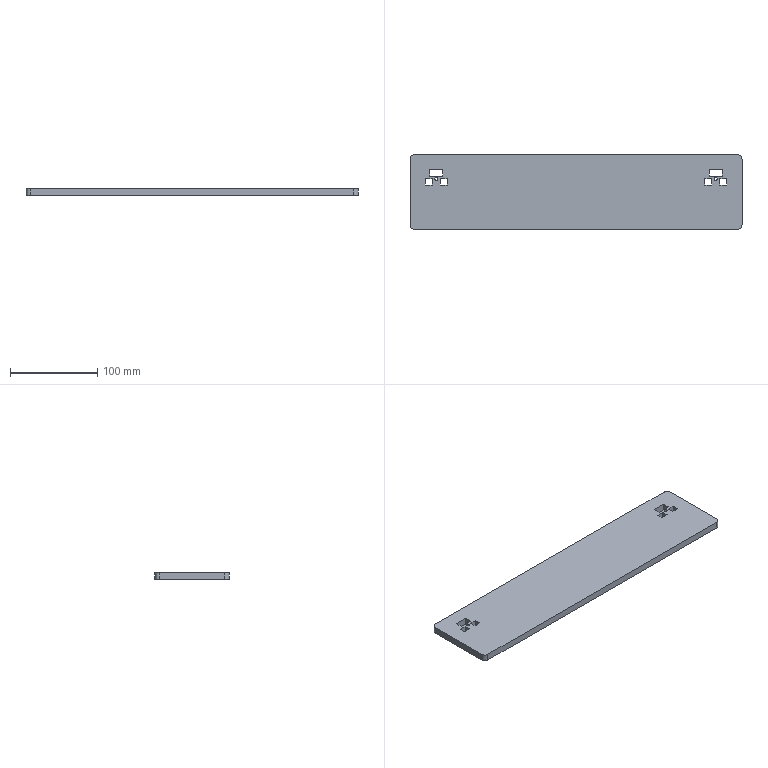Part | SolidWorks | features Fillet 1, FlatPattern 1, SMBaseFlange 1, SheetMetal 1 | 1 solid | 38 faces | box 380 x 85 x 8 mm | volume 254362 mm3 | plane 30 | cylinder 8 | commonest cylinder face diameters 3.5 x4 10 x4
STEP:
#1=CARTESIAN_POINT('',(322.8,26.043,8.));
#2=VERTEX_POINT('',#1);
#3=CARTESIAN_POINT('',(326.3,26.043,8.));
#4=VERTEX_POINT('',#3);
#5=CARTESIAN_POINT('',(324.55,26.043,8.));
#6=DIRECTION('',(0.,0.,1.));
#7=DIRECTION('',(1.,0.,0.));
#8=AXIS2_PLACEMENT_3D('',#5,#6,#7);
#9=CIRCLE('',#8,1.75);
#10=EDGE_CURVE('',#2,#4,#9,.T.);
#11=ORIENTED_EDGE('',*,*,#10,.T.);
#12=CARTESIAN_POINT('',(326.3,26.043,0.));
#13=VERTEX_POINT('',#12);
#14=CARTESIAN_POINT('',(326.3,26.043,8.));
#15=DIRECTION('',(0.,0.,-1.));
#16=VECTOR('',#15,1000.);
#17=LINE('',#14,#16);
#18=EDGE_CURVE('',#4,#13,#17,.T.);
#19=ORIENTED_EDGE('',*,*,#18,.T.);
#20=CARTESIAN_POINT('',(322.8,26.043,0.));
#21=VERTEX_POINT('',#20);
#22=CARTESIAN_POINT('',(324.55,26.043,0.));
#23=DIRECTION('',(0.,0.,1.));
#24=DIRECTION('',(1.,0.,0.));
#25=AXIS2_PLACEMENT_3D('',#22,#23,#24);
#26=CIRCLE('',#25,1.75);
#27=EDGE_CURVE('',#21,#13,#26,.T.);
#28=ORIENTED_EDGE('',*,*,#27,.F.);
#29=CARTESIAN_POINT('',(322.8,26.043,8.));
#30=DIRECTION('',(0.,0.,-1.));
#31=VECTOR('',#30,1000.);
#32=LINE('',#29,#31);
#33=EDGE_CURVE('',#2,#21,#32,.T.);
#34=ORIENTED_EDGE('',*,*,#33,.F.);
#35=EDGE_LOOP('',(#11,#19,#28,#34));
#36=FACE_OUTER_BOUND('',#35,.T.);
#37=CARTESIAN_POINT('',(324.55,26.043,8.));
#38=DIRECTION('',(0.,0.,-1.));
#39=DIRECTION('',(-1.,0.,0.));
#40=AXIS2_PLACEMENT_3D('',#37,#38,#39);
#41=CYLINDRICAL_SURFACE('',#40,1.75);
#42=ADVANCED_FACE('',(#36),#41,.F.);
#43=CARTESIAN_POINT('',(2.8,26.043,8.));
#44=VERTEX_POINT('',#43);
#45=CARTESIAN_POINT('',(6.3,26.043,8.));
#46=VERTEX_POINT('',#45);
#47=CARTESIAN_POINT('',(4.55,26.043,8.));
#48=DIRECTION('',(0.,0.,1.));
#49=DIRECTION('',(1.,0.,0.));
#50=AXIS2_PLACEMENT_3D('',#47,#48,#49);
#51=CIRCLE('',#50,1.75);
#52=EDGE_CURVE('',#44,#46,#51,.T.);
#53=ORIENTED_EDGE('',*,*,#52,.T.);
#54=CARTESIAN_POINT('',(6.3,26.043,0.));
#55=VERTEX_POINT('',#54);
#56=CARTESIAN_POINT('',(6.3,26.043,8.));
#57=DIRECTION('',(0.,0.,-1.));
#58=VECTOR('',#57,1000.);
#59=LINE('',#56,#58);
#60=EDGE_CURVE('',#46,#55,#59,.T.);
#61=ORIENTED_EDGE('',*,*,#60,.T.);
#62=CARTESIAN_POINT('',(2.8,26.043,0.));
#63=VERTEX_POINT('',#62);
#64=CARTESIAN_POINT('',(4.55,26.043,0.));
#65=DIRECTION('',(0.,0.,1.));
#66=DIRECTION('',(1.,0.,0.));
#67=AXIS2_PLACEMENT_3D('',#64,#65,#66);
#68=CIRCLE('',#67,1.75);
#69=EDGE_CURVE('',#63,#55,#68,.T.);
#70=ORIENTED_EDGE('',*,*,#69,.F.);
#71=CARTESIAN_POINT('',(2.8,26.043,8.));
#72=DIRECTION('',(0.,0.,-1.));
#73=VECTOR('',#72,1000.);
#74=LINE('',#71,#73);
#75=EDGE_CURVE('',#44,#63,#74,.T.);
#76=ORIENTED_EDGE('',*,*,#75,.F.);
#77=EDGE_LOOP('',(#53,#61,#70,#76));
#78=FACE_OUTER_BOUND('',#77,.T.);
#79=CARTESIAN_POINT('',(4.55,26.043,8.));
#80=DIRECTION('',(0.,0.,-1.));
#81=DIRECTION('',(-1.,0.,0.));
#82=AXIS2_PLACEMENT_3D('',#79,#80,#81);
#83=CYLINDRICAL_SURFACE('',#82,1.75);
#84=ADVANCED_FACE('',(#78),#83,.F.);
#85=CARTESIAN_POINT('',(320.,19.043,8.));
#86=VERTEX_POINT('',#85);
#87=CARTESIAN_POINT('',(320.,26.043,8.));
#88=VERTEX_POINT('',#87);
#89=CARTESIAN_POINT('',(320.,26.043,8.));
#90=DIRECTION('',(0.,1.,0.));
#91=VECTOR('',#90,1000.);
#92=LINE('',#89,#91);
#93=EDGE_CURVE('',#86,#88,#92,.T.);
#94=ORIENTED_EDGE('',*,*,#93,.F.);
#95=CARTESIAN_POINT('',(312.,19.043,8.));
#96=VERTEX_POINT('',#95);
#97=CARTESIAN_POINT('',(320.,19.043,8.));
#98=DIRECTION('',(1.,0.,0.));
#99=VECTOR('',#98,1000.);
#100=LINE('',#97,#99);
#101=EDGE_CURVE('',#96,#86,#100,.T.);
#102=ORIENTED_EDGE('',*,*,#101,.F.);
#103=CARTESIAN_POINT('',(312.,26.043,8.));
#104=VERTEX_POINT('',#103);
#105=CARTESIAN_POINT('',(312.,26.043,8.));
#106=DIRECTION('',(0.,-1.,0.));
#107=VECTOR('',#106,1000.);
#108=LINE('',#105,#107);
#109=EDGE_CURVE('',#104,#96,#108,.T.);
#110=ORIENTED_EDGE('',*,*,#109,.F.);
#111=CARTESIAN_POINT('',(320.,26.043,8.));
#112=DIRECTION('',(-1.,0.,0.));
#113=VECTOR('',#112,1000.);
#114=LINE('',#111,#113);
#115=EDGE_CURVE('',#88,#104,#114,.T.);
#116=ORIENTED_EDGE('',*,*,#115,.F.);
#117=EDGE_LOOP('',(#94,#102,#110,#116));
#118=FACE_BOUND('',#117,.T.);
#119=CARTESIAN_POINT('',(-8.,26.043,8.));
#120=VERTEX_POINT('',#119);
#121=CARTESIAN_POINT('',(-8.,19.043,8.));
#122=VERTEX_POINT('',#121);
#123=CARTESIAN_POINT('',(-8.,19.043,8.));
#124=DIRECTION('',(0.,-1.,0.));
#125=VECTOR('',#124,1000.);
#126=LINE('',#123,#125);
#127=EDGE_CURVE('',#120,#122,#126,.T.);
#128=ORIENTED_EDGE('',*,*,#127,.F.);
#129=CARTESIAN_POINT('',(0.,26.043,8.));
#130=VERTEX_POINT('',#129);
#131=CARTESIAN_POINT('',(-8.,26.043,8.));
#132=DIRECTION('',(-1.,0.,0.));
#133=VECTOR('',#132,1000.);
#134=LINE('',#131,#133);
#135=EDGE_CURVE('',#130,#120,#134,.T.);
#136=ORIENTED_EDGE('',*,*,#135,.F.);
#137=CARTESIAN_POINT('',(0.,19.043,8.));
#138=VERTEX_POINT('',#137);
#139=CARTESIAN_POINT('',(0.,19.043,8.));
#140=DIRECTION('',(0.,1.,0.));
#141=VECTOR('',#140,1000.);
#142=LINE('',#139,#141);
#143=EDGE_CURVE('',#138,#130,#142,.T.);
#144=ORIENTED_EDGE('',*,*,#143,.F.);
#145=CARTESIAN_POINT('',(-8.,19.043,8.));
#146=DIRECTION('',(1.,0.,0.));
#147=VECTOR('',#146,1000.);
#148=LINE('',#145,#147);
#149=EDGE_CURVE('',#122,#138,#148,.T.);
#150=ORIENTED_EDGE('',*,*,#149,.F.);
#151=EDGE_LOOP('',(#128,#136,#144,#150));
#152=FACE_BOUND('',#151,.T.);
#153=CARTESIAN_POINT('',(-2.95,37.043,8.));
#154=VERTEX_POINT('',#153);
#155=CARTESIAN_POINT('',(-2.95,29.043,8.));
#156=VERTEX_POINT('',#155);
#157=CARTESIAN_POINT('',(-2.95,29.043,8.));
#158=DIRECTION('',(0.,-1.,0.));
#159=VECTOR('',#158,1000.);
#160=LINE('',#157,#159);
#161=EDGE_CURVE('',#154,#156,#160,.T.);
#162=ORIENTED_EDGE('',*,*,#161,.F.);
#163=CARTESIAN_POINT('',(12.05,37.043,8.));
#164=VERTEX_POINT('',#163);
#165=CARTESIAN_POINT('',(-2.95,37.043,8.));
#166=DIRECTION('',(-1.,0.,0.));
#167=VECTOR('',#166,1000.);
#168=LINE('',#165,#167);
#169=EDGE_CURVE('',#164,#154,#168,.T.);
#170=ORIENTED_EDGE('',*,*,#169,.F.);
#171=CARTESIAN_POINT('',(12.05,29.043,8.));
#172=VERTEX_POINT('',#171);
#173=CARTESIAN_POINT('',(12.05,29.043,8.));
#174=DIRECTION('',(0.,1.,0.));
#175=VECTOR('',#174,1000.);
#176=LINE('',#173,#175);
#177=EDGE_CURVE('',#172,#164,#176,.T.);
#178=ORIENTED_EDGE('',*,*,#177,.F.);
#179=CARTESIAN_POINT('',(-2.95,29.043,8.));
#180=DIRECTION('',(1.,0.,0.));
#181=VECTOR('',#180,1000.);
#182=LINE('',#179,#181);
#183=EDGE_CURVE('',#156,#172,#182,.T.);
#184=ORIENTED_EDGE('',*,*,#183,.F.);
#185=EDGE_LOOP('',(#162,#170,#178,#184));
#186=FACE_BOUND('',#185,.T.);
#187=CARTESIAN_POINT('',(354.55,-26.457,8.));
#188=VERTEX_POINT('',#187);
#189=CARTESIAN_POINT('',(354.55,48.543,8.));
#190=VERTEX_POINT('',#189);
#191=CARTESIAN_POINT('',(354.55,-31.457,8.));
#192=DIRECTION('',(0.,1.,0.));
#193=VECTOR('',#192,1000.);
#194=LINE('',#191,#193);
#195=EDGE_CURVE('',#188,#190,#194,.T.);
#196=ORIENTED_EDGE('',*,*,#195,.T.);
#197=CARTESIAN_POINT('',(349.55,53.543,8.));
#198=VERTEX_POINT('',#197);
#199=CARTESIAN_POINT('',(349.55,48.543,8.));
#200=DIRECTION('',(0.,0.,1.));
#201=DIRECTION('',(-1.,0.,0.));
#202=AXIS2_PLACEMENT_3D('',#199,#200,#201);
#203=CIRCLE('',#202,5.);
#204=EDGE_CURVE('',#190,#198,#203,.T.);
#205=ORIENTED_EDGE('',*,*,#204,.T.);
#206=CARTESIAN_POINT('',(-20.45,53.543,8.));
#207=VERTEX_POINT('',#206);
#208=CARTESIAN_POINT('',(-25.45,53.543,8.));
#209=DIRECTION('',(-1.,0.,0.));
#210=VECTOR('',#209,1000.);
#211=LINE('',#208,#210);
#212=EDGE_CURVE('',#198,#207,#211,.T.);
#213=ORIENTED_EDGE('',*,*,#212,.T.);
#214=CARTESIAN_POINT('',(-25.45,48.543,8.));
#215=VERTEX_POINT('',#214);
#216=CARTESIAN_POINT('',(-20.45,48.543,8.));
#217=DIRECTION('',(0.,0.,1.));
#218=DIRECTION('',(-1.,0.,0.));
#219=AXIS2_PLACEMENT_3D('',#216,#217,#218);
#220=CIRCLE('',#219,5.);
#221=EDGE_CURVE('',#207,#215,#220,.T.);
#222=ORIENTED_EDGE('',*,*,#221,.T.);
#223=CARTESIAN_POINT('',(-25.45,-26.457,8.));
#224=VERTEX_POINT('',#223);
#225=CARTESIAN_POINT('',(-25.45,-31.457,8.));
#226=DIRECTION('',(0.,-1.,0.));
#227=VECTOR('',#226,1000.);
#228=LINE('',#225,#227);
#229=EDGE_CURVE('',#215,#224,#228,.T.);
#230=ORIENTED_EDGE('',*,*,#229,.T.);
#231=CARTESIAN_POINT('',(-20.45,-31.457,8.));
#232=VERTEX_POINT('',#231);
#233=CARTESIAN_POINT('',(-20.45,-26.457,8.));
#234=DIRECTION('',(0.,0.,1.));
#235=DIRECTION('',(-1.,0.,0.));
#236=AXIS2_PLACEMENT_3D('',#233,#234,#235);
#237=CIRCLE('',#236,5.);
#238=EDGE_CURVE('',#224,#232,#237,.T.);
#239=ORIENTED_EDGE('',*,*,#238,.T.);
#240=CARTESIAN_POINT('',(349.55,-31.457,8.));
#241=VERTEX_POINT('',#240);
#242=CARTESIAN_POINT('',(-25.45,-31.457,8.));
#243=DIRECTION('',(1.,0.,0.));
#244=VECTOR('',#243,1000.);
#245=LINE('',#242,#244);
#246=EDGE_CURVE('',#232,#241,#245,.T.);
#247=ORIENTED_EDGE('',*,*,#246,.T.);
#248=CARTESIAN_POINT('',(349.55,-26.457,8.));
#249=DIRECTION('',(0.,0.,1.));
#250=DIRECTION('',(-1.,0.,0.));
#251=AXIS2_PLACEMENT_3D('',#248,#249,#250);
#252=CIRCLE('',#251,5.);
#253=EDGE_CURVE('',#241,#188,#252,.T.);
#254=ORIENTED_EDGE('',*,*,#253,.T.);
#255=EDGE_LOOP('',(#196,#205,#213,#222,#230,#239,#247,#254));
#256=FACE_OUTER_BOUND('',#255,.T.);
#257=CARTESIAN_POINT('',(17.1,19.043,8.));
#258=VERTEX_POINT('',#257);
#259=CARTESIAN_POINT('',(17.1,26.043,8.));
#260=VERTEX_POINT('',#259);
#261=CARTESIAN_POINT('',(17.1,26.043,8.));
#262=DIRECTION('',(0.,1.,0.));
#263=VECTOR('',#262,1000.);
#264=LINE('',#261,#263);
#265=EDGE_CURVE('',#258,#260,#264,.T.);
#266=ORIENTED_EDGE('',*,*,#265,.F.);
#267=CARTESIAN_POINT('',(9.1,19.043,8.));
#268=VERTEX_POINT('',#267);
#269=CARTESIAN_POINT('',(17.1,19.043,8.));
#270=DIRECTION('',(1.,0.,0.));
#271=VECTOR('',#270,1000.);
#272=LINE('',#269,#271);
#273=EDGE_CURVE('',#268,#258,#272,.T.);
#274=ORIENTED_EDGE('',*,*,#273,.F.);
#275=CARTESIAN_POINT('',(9.1,26.043,8.));
#276=VERTEX_POINT('',#275);
#277=CARTESIAN_POINT('',(9.1,26.043,8.));
#278=DIRECTION('',(0.,-1.,0.));
#279=VECTOR('',#278,1000.);
#280=LINE('',#277,#279);
#281=EDGE_CURVE('',#276,#268,#280,.T.);
#282=ORIENTED_EDGE('',*,*,#281,.F.);
#283=CARTESIAN_POINT('',(17.1,26.043,8.));
#284=DIRECTION('',(-1.,0.,0.));
#285=VECTOR('',#284,1000.);
#286=LINE('',#283,#285);
#287=EDGE_CURVE('',#260,#276,#286,.T.);
#288=ORIENTED_EDGE('',*,*,#287,.F.);
#289=EDGE_LOOP('',(#266,#274,#282,#288));
#290=FACE_BOUND('',#289,.T.);
#291=CARTESIAN_POINT('',(332.05,29.043,8.));
#292=VERTEX_POINT('',#291);
#293=CARTESIAN_POINT('',(332.05,37.043,8.));
#294=VERTEX_POINT('',#293);
#295=CARTESIAN_POINT('',(332.05,37.043,8.));
#296=DIRECTION('',(0.,1.,0.));
#297=VECTOR('',#296,1000.);
#298=LINE('',#295,#297);
#299=EDGE_CURVE('',#292,#294,#298,.T.);
#300=ORIENTED_EDGE('',*,*,#299,.F.);
#301=CARTESIAN_POINT('',(317.05,29.043,8.));
#302=VERTEX_POINT('',#301);
#303=CARTESIAN_POINT('',(332.05,29.043,8.));
#304=DIRECTION('',(1.,0.,0.));
#305=VECTOR('',#304,1000.);
#306=LINE('',#303,#305);
#307=EDGE_CURVE('',#302,#292,#306,.T.);
#308=ORIENTED_EDGE('',*,*,#307,.F.);
#309=CARTESIAN_POINT('',(317.05,37.043,8.));
#310=VERTEX_POINT('',#309);
#311=CARTESIAN_POINT('',(317.05,37.043,8.));
#312=DIRECTION('',(0.,-1.,0.));
#313=VECTOR('',#312,1000.);
#314=LINE('',#311,#313);
#315=EDGE_CURVE('',#310,#302,#314,.T.);
#316=ORIENTED_EDGE('',*,*,#315,.F.);
#317=CARTESIAN_POINT('',(332.05,37.043,8.));
#318=DIRECTION('',(-1.,0.,0.));
#319=VECTOR('',#318,1000.);
#320=LINE('',#317,#319);
#321=EDGE_CURVE('',#294,#310,#320,.T.);
#322=ORIENTED_EDGE('',*,*,#321,.F.);
#323=EDGE_LOOP('',(#300,#308,#316,#322));
#324=FACE_BOUND('',#323,.T.);
#325=CARTESIAN_POINT('',(337.1,19.043,8.));
#326=VERTEX_POINT('',#325);
#327=CARTESIAN_POINT('',(337.1,26.043,8.));
#328=VERTEX_POINT('',#327);
#329=CARTESIAN_POINT('',(337.1,26.043,8.));
#330=DIRECTION('',(0.,1.,0.));
#331=VECTOR('',#330,1000.);
#332=LINE('',#329,#331);
#333=EDGE_CURVE('',#326,#328,#332,.T.);
#334=ORIENTED_EDGE('',*,*,#333,.F.);
#335=CARTESIAN_POINT('',(329.1,19.043,8.));
#336=VERTEX_POINT('',#335);
#337=CARTESIAN_POINT('',(337.1,19.043,8.));
#338=DIRECTION('',(1.,0.,0.));
#339=VECTOR('',#338,1000.);
#340=LINE('',#337,#339);
#341=EDGE_CURVE('',#336,#326,#340,.T.);
#342=ORIENTED_EDGE('',*,*,#341,.F.);
#343=CARTESIAN_POINT('',(329.1,26.043,8.));
#344=VERTEX_POINT('',#343);
#345=CARTESIAN_POINT('',(329.1,26.043,8.));
#346=DIRECTION('',(0.,-1.,0.));
#347=VECTOR('',#346,1000.);
#348=LINE('',#345,#347);
#349=EDGE_CURVE('',#344,#336,#348,.T.);
#350=ORIENTED_EDGE('',*,*,#349,.F.);
#351=CARTESIAN_POINT('',(337.1,26.043,8.));
#352=DIRECTION('',(-1.,0.,0.));
#353=VECTOR('',#352,1000.);
#354=LINE('',#351,#353);
#355=EDGE_CURVE('',#328,#344,#354,.T.);
#356=ORIENTED_EDGE('',*,*,#355,.F.);
#357=EDGE_LOOP('',(#334,#342,#350,#356));
#358=FACE_BOUND('',#357,.T.);
#359=ORIENTED_EDGE('',*,*,#52,.F.);
#360=CARTESIAN_POINT('',(4.55,26.043,8.));
#361=DIRECTION('',(0.,0.,1.));
#362=DIRECTION('',(1.,0.,0.));
#363=AXIS2_PLACEMENT_3D('',#360,#361,#362);
#364=CIRCLE('',#363,1.75);
#365=EDGE_CURVE('',#46,#44,#364,.T.);
#366=ORIENTED_EDGE('',*,*,#365,.F.);
#367=EDGE_LOOP('',(#359,#366));
#368=FACE_BOUND('',#367,.T.);
#369=ORIENTED_EDGE('',*,*,#10,.F.);
#370=CARTESIAN_POINT('',(324.55,26.043,8.));
#371=DIRECTION('',(0.,0.,1.));
#372=DIRECTION('',(1.,0.,0.));
#373=AXIS2_PLACEMENT_3D('',#370,#371,#372);
#374=CIRCLE('',#373,1.75);
#375=EDGE_CURVE('',#4,#2,#374,.T.);
#376=ORIENTED_EDGE('',*,*,#375,.F.);
#377=EDGE_LOOP('',(#369,#376));
#378=FACE_BOUND('',#377,.T.);
#379=CARTESIAN_POINT('',(0.,0.,8.));
#380=DIRECTION('',(0.,0.,-1.));
#381=DIRECTION('',(-1.,0.,0.));
#382=AXIS2_PLACEMENT_3D('',#379,#380,#381);
#383=PLANE('',#382);
#384=ADVANCED_FACE('',(#118,#152,#186,#256,#290,#324,#358,#368,#378),#383,.F.);
#385=ORIENTED_EDGE('',*,*,#69,.T.);
#386=CARTESIAN_POINT('',(4.55,26.043,0.));
#387=DIRECTION('',(0.,0.,1.));
#388=DIRECTION('',(1.,0.,0.));
#389=AXIS2_PLACEMENT_3D('',#386,#387,#388);
#390=CIRCLE('',#389,1.75);
#391=EDGE_CURVE('',#55,#63,#390,.T.);
#392=ORIENTED_EDGE('',*,*,#391,.T.);
#393=EDGE_LOOP('',(#385,#392));
#394=FACE_BOUND('',#393,.T.);
#395=CARTESIAN_POINT('',(349.55,53.543,0.));
#396=VERTEX_POINT('',#395);
#397=CARTESIAN_POINT('',(-20.45,53.543,0.));
#398=VERTEX_POINT('',#397);
#399=CARTESIAN_POINT('',(-25.45,53.543,0.));
#400=DIRECTION('',(-1.,0.,0.));
#401=VECTOR('',#400,1000.);
#402=LINE('',#399,#401);
#403=EDGE_CURVE('',#396,#398,#402,.T.);
#404=ORIENTED_EDGE('',*,*,#403,.F.);
#405=CARTESIAN_POINT('',(354.55,48.543,0.));
#406=VERTEX_POINT('',#405);
#407=CARTESIAN_POINT('',(349.55,48.543,0.));
#408=DIRECTION('',(0.,0.,-1.));
#409=DIRECTION('',(-1.,0.,0.));
#410=AXIS2_PLACEMENT_3D('',#407,#408,#409);
#411=CIRCLE('',#410,5.);
#412=EDGE_CURVE('',#396,#406,#411,.T.);
#413=ORIENTED_EDGE('',*,*,#412,.T.);
#414=CARTESIAN_POINT('',(354.55,-26.457,0.));
#415=VERTEX_POINT('',#414);
#416=CARTESIAN_POINT('',(354.55,-31.457,0.));
#417=DIRECTION('',(0.,1.,0.));
#418=VECTOR('',#417,1000.);
#419=LINE('',#416,#418);
#420=EDGE_CURVE('',#415,#406,#419,.T.);
#421=ORIENTED_EDGE('',*,*,#420,.F.);
#422=CARTESIAN_POINT('',(349.55,-31.457,0.));
#423=VERTEX_POINT('',#422);
#424=CARTESIAN_POINT('',(349.55,-26.457,0.));
#425=DIRECTION('',(0.,0.,-1.));
#426=DIRECTION('',(-1.,0.,0.));
#427=AXIS2_PLACEMENT_3D('',#424,#425,#426);
#428=CIRCLE('',#427,5.);
#429=EDGE_CURVE('',#415,#423,#428,.T.);
#430=ORIENTED_EDGE('',*,*,#429,.T.);
#431=CARTESIAN_POINT('',(-20.45,-31.457,0.));
#432=VERTEX_POINT('',#431);
#433=CARTESIAN_POINT('',(-25.45,-31.457,0.));
#434=DIRECTION('',(1.,0.,0.));
#435=VECTOR('',#434,1000.);
#436=LINE('',#433,#435);
#437=EDGE_CURVE('',#432,#423,#436,.T.);
#438=ORIENTED_EDGE('',*,*,#437,.F.);
#439=CARTESIAN_POINT('',(-25.45,-26.457,0.));
#440=VERTEX_POINT('',#439);
#441=CARTESIAN_POINT('',(-20.45,-26.457,0.));
#442=DIRECTION('',(0.,0.,-1.));
#443=DIRECTION('',(-1.,0.,0.));
#444=AXIS2_PLACEMENT_3D('',#441,#442,#443);
#445=CIRCLE('',#444,5.);
#446=EDGE_CURVE('',#432,#440,#445,.T.);
#447=ORIENTED_EDGE('',*,*,#446,.T.);
#448=CARTESIAN_POINT('',(-25.45,48.543,0.));
#449=VERTEX_POINT('',#448);
#450=CARTESIAN_POINT('',(-25.45,-31.457,0.));
#451=DIRECTION('',(0.,-1.,0.));
#452=VECTOR('',#451,1000.);
#453=LINE('',#450,#452);
#454=EDGE_CURVE('',#449,#440,#453,.T.);
#455=ORIENTED_EDGE('',*,*,#454,.F.);
#456=CARTESIAN_POINT('',(-20.45,48.543,0.));
#457=DIRECTION('',(0.,0.,-1.));
#458=DIRECTION('',(-1.,0.,0.));
#459=AXIS2_PLACEMENT_3D('',#456,#457,#458);
#460=CIRCLE('',#459,5.);
#461=EDGE_CURVE('',#449,#398,#460,.T.);
#462=ORIENTED_EDGE('',*,*,#461,.T.);
#463=EDGE_LOOP('',(#404,#413,#421,#430,#438,#447,#455,#462));
#464=FACE_OUTER_BOUND('',#463,.T.);
#465=CARTESIAN_POINT('',(12.05,37.043,0.));
#466=VERTEX_POINT('',#465);
#467=CARTESIAN_POINT('',(-2.95,37.043,0.));
#468=VERTEX_POINT('',#467);
#469=CARTESIAN_POINT('',(-2.95,37.043,0.));
#470=DIRECTION('',(-1.,0.,0.));
#471=VECTOR('',#470,1000.);
#472=LINE('',#469,#471);
#473=EDGE_CURVE('',#466,#468,#472,.T.);
#474=ORIENTED_EDGE('',*,*,#473,.T.);
#475=CARTESIAN_POINT('',(-2.95,29.043,0.));
#476=VERTEX_POINT('',#475);
#477=CARTESIAN_POINT('',(-2.95,29.043,0.));
#478=DIRECTION('',(0.,-1.,0.));
#479=VECTOR('',#478,1000.);
#480=LINE('',#477,#479);
#481=EDGE_CURVE('',#468,#476,#480,.T.);
#482=ORIENTED_EDGE('',*,*,#481,.T.);
#483=CARTESIAN_POINT('',(12.05,29.043,0.));
#484=VERTEX_POINT('',#483);
#485=CARTESIAN_POINT('',(-2.95,29.043,0.));
#486=DIRECTION('',(1.,0.,0.));
#487=VECTOR('',#486,1000.);
#488=LINE('',#485,#487);
#489=EDGE_CURVE('',#476,#484,#488,.T.);
#490=ORIENTED_EDGE('',*,*,#489,.T.);
#491=CARTESIAN_POINT('',(12.05,29.043,0.));
#492=DIRECTION('',(0.,1.,0.));
#493=VECTOR('',#492,1000.);
#494=LINE('',#491,#493);
#495=EDGE_CURVE('',#484,#466,#494,.T.);
#496=ORIENTED_EDGE('',*,*,#495,.T.);
#497=EDGE_LOOP('',(#474,#482,#490,#496));
#498=FACE_BOUND('',#497,.T.);
#499=CARTESIAN_POINT('',(9.1,19.043,0.));
#500=VERTEX_POINT('',#499);
#501=CARTESIAN_POINT('',(17.1,19.043,0.));
#502=VERTEX_POINT('',#501);
#503=CARTESIAN_POINT('',(17.1,19.043,0.));
#504=DIRECTION('',(1.,0.,0.));
#505=VECTOR('',#504,1000.);
#506=LINE('',#503,#505);
#507=EDGE_CURVE('',#500,#502,#506,.T.);
#508=ORIENTED_EDGE('',*,*,#507,.T.);
#509=CARTESIAN_POINT('',(17.1,26.043,0.));
#510=VERTEX_POINT('',#509);
#511=CARTESIAN_POINT('',(17.1,26.043,0.));
#512=DIRECTION('',(0.,1.,0.));
#513=VECTOR('',#512,1000.);
#514=LINE('',#511,#513);
#515=EDGE_CURVE('',#502,#510,#514,.T.);
#516=ORIENTED_EDGE('',*,*,#515,.T.);
#517=CARTESIAN_POINT('',(9.1,26.043,0.));
#518=VERTEX_POINT('',#517);
#519=CARTESIAN_POINT('',(17.1,26.043,0.));
#520=DIRECTION('',(-1.,0.,0.));
#521=VECTOR('',#520,1000.);
#522=LINE('',#519,#521);
#523=EDGE_CURVE('',#510,#518,#522,.T.);
#524=ORIENTED_EDGE('',*,*,#523,.T.);
#525=CARTESIAN_POINT('',(9.1,26.043,0.));
#526=DIRECTION('',(0.,-1.,0.));
#527=VECTOR('',#526,1000.);
#528=LINE('',#525,#527);
#529=EDGE_CURVE('',#518,#500,#528,.T.);
#530=ORIENTED_EDGE('',*,*,#529,.T.);
#531=EDGE_LOOP('',(#508,#516,#524,#530));
#532=FACE_BOUND('',#531,.T.);
#533=CARTESIAN_POINT('',(0.,26.043,0.));
#534=VERTEX_POINT('',#533);
#535=CARTESIAN_POINT('',(-8.,26.043,0.));
#536=VERTEX_POINT('',#535);
#537=CARTESIAN_POINT('',(-8.,26.043,0.));
#538=DIRECTION('',(-1.,0.,0.));
#539=VECTOR('',#538,1000.);
#540=LINE('',#537,#539);
#541=EDGE_CURVE('',#534,#536,#540,.T.);
#542=ORIENTED_EDGE('',*,*,#541,.T.);
#543=CARTESIAN_POINT('',(-8.,19.043,0.));
#544=VERTEX_POINT('',#543);
#545=CARTESIAN_POINT('',(-8.,19.043,0.));
#546=DIRECTION('',(0.,-1.,0.));
#547=VECTOR('',#546,1000.);
#548=LINE('',#545,#547);
#549=EDGE_CURVE('',#536,#544,#548,.T.);
#550=ORIENTED_EDGE('',*,*,#549,.T.);
#551=CARTESIAN_POINT('',(0.,19.043,0.));
#552=VERTEX_POINT('',#551);
#553=CARTESIAN_POINT('',(-8.,19.043,0.));
#554=DIRECTION('',(1.,0.,0.));
#555=VECTOR('',#554,1000.);
#556=LINE('',#553,#555);
#557=EDGE_CURVE('',#544,#552,#556,.T.);
#558=ORIENTED_EDGE('',*,*,#557,.T.);
#559=CARTESIAN_POINT('',(0.,19.043,0.));
#560=DIRECTION('',(0.,1.,0.));
#561=VECTOR('',#560,1000.);
#562=LINE('',#559,#561);
#563=EDGE_CURVE('',#552,#534,#562,.T.);
#564=ORIENTED_EDGE('',*,*,#563,.T.);
#565=EDGE_LOOP('',(#542,#550,#558,#564));
#566=FACE_BOUND('',#565,.T.);
#567=CARTESIAN_POINT('',(317.05,29.043,0.));
#568=VERTEX_POINT('',#567);
#569=CARTESIAN_POINT('',(332.05,29.043,0.));
#570=VERTEX_POINT('',#569);
#571=CARTESIAN_POINT('',(332.05,29.043,0.));
#572=DIRECTION('',(1.,0.,0.));
#573=VECTOR('',#572,1000.);
#574=LINE('',#571,#573);
#575=EDGE_CURVE('',#568,#570,#574,.T.);
#576=ORIENTED_EDGE('',*,*,#575,.T.);
#577=CARTESIAN_POINT('',(332.05,37.043,0.));
#578=VERTEX_POINT('',#577);
#579=CARTESIAN_POINT('',(332.05,37.043,0.));
#580=DIRECTION('',(0.,1.,0.));
#581=VECTOR('',#580,1000.);
#582=LINE('',#579,#581);
#583=EDGE_CURVE('',#570,#578,#582,.T.);
#584=ORIENTED_EDGE('',*,*,#583,.T.);
#585=CARTESIAN_POINT('',(317.05,37.043,0.));
#586=VERTEX_POINT('',#585);
#587=CARTESIAN_POINT('',(332.05,37.043,0.));
#588=DIRECTION('',(-1.,0.,0.));
#589=VECTOR('',#588,1000.);
#590=LINE('',#587,#589);
#591=EDGE_CURVE('',#578,#586,#590,.T.);
#592=ORIENTED_EDGE('',*,*,#591,.T.);
#593=CARTESIAN_POINT('',(317.05,37.043,0.));
#594=DIRECTION('',(0.,-1.,0.));
#595=VECTOR('',#594,1000.);
#596=LINE('',#593,#595);
#597=EDGE_CURVE('',#586,#568,#596,.T.);
#598=ORIENTED_EDGE('',*,*,#597,.T.);
#599=EDGE_LOOP('',(#576,#584,#592,#598));
#600=FACE_BOUND('',#599,.T.);
#601=CARTESIAN_POINT('',(312.,19.043,0.));
#602=VERTEX_POINT('',#601);
#603=CARTESIAN_POINT('',(320.,19.043,0.));
#604=VERTEX_POINT('',#603);
#605=CARTESIAN_POINT('',(320.,19.043,0.));
#606=DIRECTION('',(1.,0.,0.));
#607=VECTOR('',#606,1000.);
#608=LINE('',#605,#607);
#609=EDGE_CURVE('',#602,#604,#608,.T.);
#610=ORIENTED_EDGE('',*,*,#609,.T.);
#611=CARTESIAN_POINT('',(320.,26.043,0.));
#612=VERTEX_POINT('',#611);
#613=CARTESIAN_POINT('',(320.,26.043,0.));
#614=DIRECTION('',(0.,1.,0.));
#615=VECTOR('',#614,1000.);
#616=LINE('',#613,#615);
#617=EDGE_CURVE('',#604,#612,#616,.T.);
#618=ORIENTED_EDGE('',*,*,#617,.T.);
#619=CARTESIAN_POINT('',(312.,26.043,0.));
#620=VERTEX_POINT('',#619);
#621=CARTESIAN_POINT('',(320.,26.043,0.));
#622=DIRECTION('',(-1.,0.,0.));
#623=VECTOR('',#622,1000.);
#624=LINE('',#621,#623);
#625=EDGE_CURVE('',#612,#620,#624,.T.);
#626=ORIENTED_EDGE('',*,*,#625,.T.);
#627=CARTESIAN_POINT('',(312.,26.043,0.));
#628=DIRECTION('',(0.,-1.,0.));
#629=VECTOR('',#628,1000.);
#630=LINE('',#627,#629);
#631=EDGE_CURVE('',#620,#602,#630,.T.);
#632=ORIENTED_EDGE('',*,*,#631,.T.);
#633=EDGE_LOOP('',(#610,#618,#626,#632));
#634=FACE_BOUND('',#633,.T.);
#635=CARTESIAN_POINT('',(329.1,19.043,0.));
#636=VERTEX_POINT('',#635);
#637=CARTESIAN_POINT('',(337.1,19.043,0.));
#638=VERTEX_POINT('',#637);
#639=CARTESIAN_POINT('',(337.1,19.043,0.));
#640=DIRECTION('',(1.,0.,0.));
#641=VECTOR('',#640,1000.);
#642=LINE('',#639,#641);
#643=EDGE_CURVE('',#636,#638,#642,.T.);
#644=ORIENTED_EDGE('',*,*,#643,.T.);
#645=CARTESIAN_POINT('',(337.1,26.043,0.));
#646=VERTEX_POINT('',#645);
#647=CARTESIAN_POINT('',(337.1,26.043,0.));
#648=DIRECTION('',(0.,1.,0.));
#649=VECTOR('',#648,1000.);
#650=LINE('',#647,#649);
#651=EDGE_CURVE('',#638,#646,#650,.T.);
#652=ORIENTED_EDGE('',*,*,#651,.T.);
#653=CARTESIAN_POINT('',(329.1,26.043,0.));
#654=VERTEX_POINT('',#653);
#655=CARTESIAN_POINT('',(337.1,26.043,0.));
#656=DIRECTION('',(-1.,0.,0.));
#657=VECTOR('',#656,1000.);
#658=LINE('',#655,#657);
#659=EDGE_CURVE('',#646,#654,#658,.T.);
#660=ORIENTED_EDGE('',*,*,#659,.T.);
#661=CARTESIAN_POINT('',(329.1,26.043,0.));
#662=DIRECTION('',(0.,-1.,0.));
#663=VECTOR('',#662,1000.);
#664=LINE('',#661,#663);
#665=EDGE_CURVE('',#654,#636,#664,.T.);
#666=ORIENTED_EDGE('',*,*,#665,.T.);
#667=EDGE_LOOP('',(#644,#652,#660,#666));
#668=FACE_BOUND('',#667,.T.);
#669=ORIENTED_EDGE('',*,*,#27,.T.);
#670=CARTESIAN_POINT('',(324.55,26.043,0.));
#671=DIRECTION('',(0.,0.,1.));
#672=DIRECTION('',(1.,0.,0.));
#673=AXIS2_PLACEMENT_3D('',#670,#671,#672);
#674=CIRCLE('',#673,1.75);
#675=EDGE_CURVE('',#13,#21,#674,.T.);
#676=ORIENTED_EDGE('',*,*,#675,.T.);
#677=EDGE_LOOP('',(#669,#676));
#678=FACE_BOUND('',#677,.T.);
#679=CARTESIAN_POINT('',(0.,0.,0.));
#680=DIRECTION('',(0.,0.,-1.));
#681=DIRECTION('',(-1.,0.,0.));
#682=AXIS2_PLACEMENT_3D('',#679,#680,#681);
#683=PLANE('',#682);
#684=ADVANCED_FACE('',(#394,#464,#498,#532,#566,#600,#634,#668,#678),#683,.T.);
#685=ORIENTED_EDGE('',*,*,#420,.T.);
#686=CARTESIAN_POINT('',(354.55,48.543,8.));
#687=DIRECTION('',(0.,0.,1.));
#688=VECTOR('',#687,1000.);
#689=LINE('',#686,#688);
#690=EDGE_CURVE('',#406,#190,#689,.T.);
#691=ORIENTED_EDGE('',*,*,#690,.T.);
#692=ORIENTED_EDGE('',*,*,#195,.F.);
#693=CARTESIAN_POINT('',(354.55,-26.457,8.));
#694=DIRECTION('',(0.,0.,-1.));
#695=VECTOR('',#694,1000.);
#696=LINE('',#693,#695);
#697=EDGE_CURVE('',#188,#415,#696,.T.);
#698=ORIENTED_EDGE('',*,*,#697,.T.);
#699=EDGE_LOOP('',(#685,#691,#692,#698));
#700=FACE_OUTER_BOUND('',#699,.T.);
#701=CARTESIAN_POINT('',(354.55,-31.457,8.));
#702=DIRECTION('',(-1.,0.,0.));
#703=DIRECTION('',(0.,0.,1.));
#704=AXIS2_PLACEMENT_3D('',#701,#702,#703);
#705=PLANE('',#704);
#706=ADVANCED_FACE('',(#700),#705,.F.);
#707=ORIENTED_EDGE('',*,*,#212,.F.);
#708=CARTESIAN_POINT('',(349.55,53.543,8.));
#709=DIRECTION('',(0.,0.,-1.));
#710=VECTOR('',#709,1000.);
#711=LINE('',#708,#710);
#712=EDGE_CURVE('',#198,#396,#711,.T.);
#713=ORIENTED_EDGE('',*,*,#712,.T.);
#714=ORIENTED_EDGE('',*,*,#403,.T.);
#715=CARTESIAN_POINT('',(-20.45,53.543,8.));
#716=DIRECTION('',(0.,0.,1.));
#717=VECTOR('',#716,1000.);
#718=LINE('',#715,#717);
#719=EDGE_CURVE('',#398,#207,#718,.T.);
#720=ORIENTED_EDGE('',*,*,#719,.T.);
#721=EDGE_LOOP('',(#707,#713,#714,#720));
#722=FACE_OUTER_BOUND('',#721,.T.);
#723=CARTESIAN_POINT('',(-25.45,53.543,8.));
#724=DIRECTION('',(0.,-1.,0.));
#725=DIRECTION('',(0.,0.,-1.));
#726=AXIS2_PLACEMENT_3D('',#723,#724,#725);
#727=PLANE('',#726);
#728=ADVANCED_FACE('',(#722),#727,.F.);
#729=ORIENTED_EDGE('',*,*,#229,.F.);
#730=CARTESIAN_POINT('',(-25.45,48.543,8.));
#731=DIRECTION('',(0.,0.,-1.));
#732=VECTOR('',#731,1000.);
#733=LINE('',#730,#732);
#734=EDGE_CURVE('',#215,#449,#733,.T.);
#735=ORIENTED_EDGE('',*,*,#734,.T.);
#736=ORIENTED_EDGE('',*,*,#454,.T.);
#737=CARTESIAN_POINT('',(-25.45,-26.457,8.));
#738=DIRECTION('',(0.,0.,1.));
#739=VECTOR('',#738,1000.);
#740=LINE('',#737,#739);
#741=EDGE_CURVE('',#440,#224,#740,.T.);
#742=ORIENTED_EDGE('',*,*,#741,.T.);
#743=EDGE_LOOP('',(#729,#735,#736,#742));
#744=FACE_OUTER_BOUND('',#743,.T.);
#745=CARTESIAN_POINT('',(-25.45,-31.457,8.));
#746=DIRECTION('',(1.,0.,0.));
#747=DIRECTION('',(0.,0.,-1.));
#748=AXIS2_PLACEMENT_3D('',#745,#746,#747);
#749=PLANE('',#748);
#750=ADVANCED_FACE('',(#744),#749,.F.);
#751=ORIENTED_EDGE('',*,*,#437,.T.);
#752=CARTESIAN_POINT('',(349.55,-31.457,8.));
#753=DIRECTION('',(0.,0.,1.));
#754=VECTOR('',#753,1000.);
#755=LINE('',#752,#754);
#756=EDGE_CURVE('',#423,#241,#755,.T.);
#757=ORIENTED_EDGE('',*,*,#756,.T.);
#758=ORIENTED_EDGE('',*,*,#246,.F.);
#759=CARTESIAN_POINT('',(-20.45,-31.457,8.));
#760=DIRECTION('',(0.,0.,-1.));
#761=VECTOR('',#760,1000.);
#762=LINE('',#759,#761);
#763=EDGE_CURVE('',#232,#432,#762,.T.);
#764=ORIENTED_EDGE('',*,*,#763,.T.);
#765=EDGE_LOOP('',(#751,#757,#758,#764));
#766=FACE_OUTER_BOUND('',#765,.T.);
#767=CARTESIAN_POINT('',(-25.45,-31.457,8.));
#768=DIRECTION('',(0.,1.,0.));
#769=DIRECTION('',(0.,0.,1.));
#770=AXIS2_PLACEMENT_3D('',#767,#768,#769);
#771=PLANE('',#770);
#772=ADVANCED_FACE('',(#766),#771,.F.);
#773=ORIENTED_EDGE('',*,*,#481,.F.);
#774=CARTESIAN_POINT('',(-2.95,37.043,8.));
#775=DIRECTION('',(0.,0.,-1.));
#776=VECTOR('',#775,1000.);
#777=LINE('',#774,#776);
#778=EDGE_CURVE('',#154,#468,#777,.T.);
#779=ORIENTED_EDGE('',*,*,#778,.F.);
#780=ORIENTED_EDGE('',*,*,#161,.T.);
#781=CARTESIAN_POINT('',(-2.95,29.043,8.));
#782=DIRECTION('',(0.,0.,-1.));
#783=VECTOR('',#782,1000.);
#784=LINE('',#781,#783);
#785=EDGE_CURVE('',#156,#476,#784,.T.);
#786=ORIENTED_EDGE('',*,*,#785,.T.);
#787=EDGE_LOOP('',(#773,#779,#780,#786));
#788=FACE_OUTER_BOUND('',#787,.T.);
#789=CARTESIAN_POINT('',(-2.95,29.043,8.));
#790=DIRECTION('',(1.,0.,0.));
#791=DIRECTION('',(0.,0.,-1.));
#792=AXIS2_PLACEMENT_3D('',#789,#790,#791);
#793=PLANE('',#792);
#794=ADVANCED_FACE('',(#788),#793,.T.);
#795=ORIENTED_EDGE('',*,*,#489,.F.);
#796=ORIENTED_EDGE('',*,*,#785,.F.);
#797=ORIENTED_EDGE('',*,*,#183,.T.);
#798=CARTESIAN_POINT('',(12.05,29.043,8.));
#799=DIRECTION('',(0.,0.,-1.));
#800=VECTOR('',#799,1000.);
#801=LINE('',#798,#800);
#802=EDGE_CURVE('',#172,#484,#801,.T.);
#803=ORIENTED_EDGE('',*,*,#802,.T.);
#804=EDGE_LOOP('',(#795,#796,#797,#803));
#805=FACE_OUTER_BOUND('',#804,.T.);
#806=CARTESIAN_POINT('',(-2.95,29.043,8.));
#807=DIRECTION('',(0.,1.,0.));
#808=DIRECTION('',(0.,0.,1.));
#809=AXIS2_PLACEMENT_3D('',#806,#807,#808);
#810=PLANE('',#809);
#811=ADVANCED_FACE('',(#805),#810,.T.);
#812=ORIENTED_EDGE('',*,*,#495,.F.);
#813=ORIENTED_EDGE('',*,*,#802,.F.);
#814=ORIENTED_EDGE('',*,*,#177,.T.);
#815=CARTESIAN_POINT('',(12.05,37.043,8.));
#816=DIRECTION('',(0.,0.,-1.));
#817=VECTOR('',#816,1000.);
#818=LINE('',#815,#817);
#819=EDGE_CURVE('',#164,#466,#818,.T.);
#820=ORIENTED_EDGE('',*,*,#819,.T.);
#821=EDGE_LOOP('',(#812,#813,#814,#820));
#822=FACE_OUTER_BOUND('',#821,.T.);
#823=CARTESIAN_POINT('',(12.05,29.043,8.));
#824=DIRECTION('',(-1.,0.,0.));
#825=DIRECTION('',(0.,0.,1.));
#826=AXIS2_PLACEMENT_3D('',#823,#824,#825);
#827=PLANE('',#826);
#828=ADVANCED_FACE('',(#822),#827,.T.);
#829=ORIENTED_EDGE('',*,*,#473,.F.);
#830=ORIENTED_EDGE('',*,*,#819,.F.);
#831=ORIENTED_EDGE('',*,*,#169,.T.);
#832=ORIENTED_EDGE('',*,*,#778,.T.);
#833=EDGE_LOOP('',(#829,#830,#831,#832));
#834=FACE_OUTER_BOUND('',#833,.T.);
#835=CARTESIAN_POINT('',(-2.95,37.043,8.));
#836=DIRECTION('',(0.,-1.,0.));
#837=DIRECTION('',(0.,0.,-1.));
#838=AXIS2_PLACEMENT_3D('',#835,#836,#837);
#839=PLANE('',#838);
#840=ADVANCED_FACE('',(#834),#839,.T.);
#841=ORIENTED_EDGE('',*,*,#515,.F.);
#842=CARTESIAN_POINT('',(17.1,19.043,8.));
#843=DIRECTION('',(0.,0.,-1.));
#844=VECTOR('',#843,1000.);
#845=LINE('',#842,#844);
#846=EDGE_CURVE('',#258,#502,#845,.T.);
#847=ORIENTED_EDGE('',*,*,#846,.F.);
#848=ORIENTED_EDGE('',*,*,#265,.T.);
#849=CARTESIAN_POINT('',(17.1,26.043,8.));
#850=DIRECTION('',(0.,0.,-1.));
#851=VECTOR('',#850,1000.);
#852=LINE('',#849,#851);
#853=EDGE_CURVE('',#260,#510,#852,.T.);
#854=ORIENTED_EDGE('',*,*,#853,.T.);
#855=EDGE_LOOP('',(#841,#847,#848,#854));
#856=FACE_OUTER_BOUND('',#855,.T.);
#857=CARTESIAN_POINT('',(17.1,26.043,8.));
#858=DIRECTION('',(-1.,0.,0.));
#859=DIRECTION('',(0.,0.,1.));
#860=AXIS2_PLACEMENT_3D('',#857,#858,#859);
#861=PLANE('',#860);
#862=ADVANCED_FACE('',(#856),#861,.T.);
#863=ORIENTED_EDGE('',*,*,#523,.F.);
#864=ORIENTED_EDGE('',*,*,#853,.F.);
#865=ORIENTED_EDGE('',*,*,#287,.T.);
#866=CARTESIAN_POINT('',(9.1,26.043,8.));
#867=DIRECTION('',(0.,0.,-1.));
#868=VECTOR('',#867,1000.);
#869=LINE('',#866,#868);
#870=EDGE_CURVE('',#276,#518,#869,.T.);
#871=ORIENTED_EDGE('',*,*,#870,.T.);
#872=EDGE_LOOP('',(#863,#864,#865,#871));
#873=FACE_OUTER_BOUND('',#872,.T.);
#874=CARTESIAN_POINT('',(17.1,26.043,8.));
#875=DIRECTION('',(0.,-1.,0.));
#876=DIRECTION('',(0.,0.,-1.));
#877=AXIS2_PLACEMENT_3D('',#874,#875,#876);
#878=PLANE('',#877);
#879=ADVANCED_FACE('',(#873),#878,.T.);
#880=ORIENTED_EDGE('',*,*,#529,.F.);
#881=ORIENTED_EDGE('',*,*,#870,.F.);
#882=ORIENTED_EDGE('',*,*,#281,.T.);
#883=CARTESIAN_POINT('',(9.1,19.043,8.));
#884=DIRECTION('',(0.,0.,-1.));
#885=VECTOR('',#884,1000.);
#886=LINE('',#883,#885);
#887=EDGE_CURVE('',#268,#500,#886,.T.);
#888=ORIENTED_EDGE('',*,*,#887,.T.);
#889=EDGE_LOOP('',(#880,#881,#882,#888));
#890=FACE_OUTER_BOUND('',#889,.T.);
#891=CARTESIAN_POINT('',(9.1,26.043,8.));
#892=DIRECTION('',(1.,0.,0.));
#893=DIRECTION('',(0.,0.,-1.));
#894=AXIS2_PLACEMENT_3D('',#891,#892,#893);
#895=PLANE('',#894);
#896=ADVANCED_FACE('',(#890),#895,.T.);
#897=ORIENTED_EDGE('',*,*,#507,.F.);
#898=ORIENTED_EDGE('',*,*,#887,.F.);
#899=ORIENTED_EDGE('',*,*,#273,.T.);
#900=ORIENTED_EDGE('',*,*,#846,.T.);
#901=EDGE_LOOP('',(#897,#898,#899,#900));
#902=FACE_OUTER_BOUND('',#901,.T.);
#903=CARTESIAN_POINT('',(17.1,19.043,8.));
#904=DIRECTION('',(0.,1.,0.));
#905=DIRECTION('',(0.,0.,1.));
#906=AXIS2_PLACEMENT_3D('',#903,#904,#905);
#907=PLANE('',#906);
#908=ADVANCED_FACE('',(#902),#907,.T.);
#909=ORIENTED_EDGE('',*,*,#549,.F.);
#910=CARTESIAN_POINT('',(-8.,26.043,8.));
#911=DIRECTION('',(0.,0.,-1.));
#912=VECTOR('',#911,1000.);
#913=LINE('',#910,#912);
#914=EDGE_CURVE('',#120,#536,#913,.T.);
#915=ORIENTED_EDGE('',*,*,#914,.F.);
#916=ORIENTED_EDGE('',*,*,#127,.T.);
#917=CARTESIAN_POINT('',(-8.,19.043,8.));
#918=DIRECTION('',(0.,0.,-1.));
#919=VECTOR('',#918,1000.);
#920=LINE('',#917,#919);
#921=EDGE_CURVE('',#122,#544,#920,.T.);
#922=ORIENTED_EDGE('',*,*,#921,.T.);
#923=EDGE_LOOP('',(#909,#915,#916,#922));
#924=FACE_OUTER_BOUND('',#923,.T.);
#925=CARTESIAN_POINT('',(-8.,19.043,8.));
#926=DIRECTION('',(1.,0.,0.));
#927=DIRECTION('',(0.,0.,-1.));
#928=AXIS2_PLACEMENT_3D('',#925,#926,#927);
#929=PLANE('',#928);
#930=ADVANCED_FACE('',(#924),#929,.T.);
#931=ORIENTED_EDGE('',*,*,#557,.F.);
#932=ORIENTED_EDGE('',*,*,#921,.F.);
#933=ORIENTED_EDGE('',*,*,#149,.T.);
#934=CARTESIAN_POINT('',(0.,19.043,8.));
#935=DIRECTION('',(0.,0.,-1.));
#936=VECTOR('',#935,1000.);
#937=LINE('',#934,#936);
#938=EDGE_CURVE('',#138,#552,#937,.T.);
#939=ORIENTED_EDGE('',*,*,#938,.T.);
#940=EDGE_LOOP('',(#931,#932,#933,#939));
#941=FACE_OUTER_BOUND('',#940,.T.);
#942=CARTESIAN_POINT('',(-8.,19.043,8.));
#943=DIRECTION('',(0.,1.,0.));
#944=DIRECTION('',(0.,0.,1.));
#945=AXIS2_PLACEMENT_3D('',#942,#943,#944);
#946=PLANE('',#945);
#947=ADVANCED_FACE('',(#941),#946,.T.);
#948=ORIENTED_EDGE('',*,*,#563,.F.);
#949=ORIENTED_EDGE('',*,*,#938,.F.);
#950=ORIENTED_EDGE('',*,*,#143,.T.);
#951=CARTESIAN_POINT('',(0.,26.043,8.));
#952=DIRECTION('',(0.,0.,-1.));
#953=VECTOR('',#952,1000.);
#954=LINE('',#951,#953);
#955=EDGE_CURVE('',#130,#534,#954,.T.);
#956=ORIENTED_EDGE('',*,*,#955,.T.);
#957=EDGE_LOOP('',(#948,#949,#950,#956));
#958=FACE_OUTER_BOUND('',#957,.T.);
#959=CARTESIAN_POINT('',(0.,19.043,8.));
#960=DIRECTION('',(-1.,0.,0.));
#961=DIRECTION('',(0.,0.,1.));
#962=AXIS2_PLACEMENT_3D('',#959,#960,#961);
#963=PLANE('',#962);
#964=ADVANCED_FACE('',(#958),#963,.T.);
#965=ORIENTED_EDGE('',*,*,#541,.F.);
#966=ORIENTED_EDGE('',*,*,#955,.F.);
#967=ORIENTED_EDGE('',*,*,#135,.T.);
#968=ORIENTED_EDGE('',*,*,#914,.T.);
#969=EDGE_LOOP('',(#965,#966,#967,#968));
#970=FACE_OUTER_BOUND('',#969,.T.);
#971=CARTESIAN_POINT('',(-8.,26.043,8.));
#972=DIRECTION('',(0.,-1.,0.));
#973=DIRECTION('',(0.,0.,-1.));
#974=AXIS2_PLACEMENT_3D('',#971,#972,#973);
#975=PLANE('',#974);
#976=ADVANCED_FACE('',(#970),#975,.T.);
#977=ORIENTED_EDGE('',*,*,#583,.F.);
#978=CARTESIAN_POINT('',(332.05,29.043,8.));
#979=DIRECTION('',(0.,0.,-1.));
#980=VECTOR('',#979,1000.);
#981=LINE('',#978,#980);
#982=EDGE_CURVE('',#292,#570,#981,.T.);
#983=ORIENTED_EDGE('',*,*,#982,.F.);
#984=ORIENTED_EDGE('',*,*,#299,.T.);
#985=CARTESIAN_POINT('',(332.05,37.043,8.));
#986=DIRECTION('',(0.,0.,-1.));
#987=VECTOR('',#986,1000.);
#988=LINE('',#985,#987);
#989=EDGE_CURVE('',#294,#578,#988,.T.);
#990=ORIENTED_EDGE('',*,*,#989,.T.);
#991=EDGE_LOOP('',(#977,#983,#984,#990));
#992=FACE_OUTER_BOUND('',#991,.T.);
#993=CARTESIAN_POINT('',(332.05,37.043,8.));
#994=DIRECTION('',(-1.,0.,0.));
#995=DIRECTION('',(0.,0.,1.));
#996=AXIS2_PLACEMENT_3D('',#993,#994,#995);
#997=PLANE('',#996);
#998=ADVANCED_FACE('',(#992),#997,.T.);
#999=ORIENTED_EDGE('',*,*,#591,.F.);
#1000=ORIENTED_EDGE('',*,*,#989,.F.);
#1001=ORIENTED_EDGE('',*,*,#321,.T.);
#1002=CARTESIAN_POINT('',(317.05,37.043,8.));
#1003=DIRECTION('',(0.,0.,-1.));
#1004=VECTOR('',#1003,1000.);
#1005=LINE('',#1002,#1004);
#1006=EDGE_CURVE('',#310,#586,#1005,.T.);
#1007=ORIENTED_EDGE('',*,*,#1006,.T.);
#1008=EDGE_LOOP('',(#999,#1000,#1001,#1007));
#1009=FACE_OUTER_BOUND('',#1008,.T.);
#1010=CARTESIAN_POINT('',(332.05,37.043,8.));
#1011=DIRECTION('',(0.,-1.,0.));
#1012=DIRECTION('',(0.,0.,-1.));
#1013=AXIS2_PLACEMENT_3D('',#1010,#1011,#1012);
#1014=PLANE('',#1013);
#1015=ADVANCED_FACE('',(#1009),#1014,.T.);
#1016=ORIENTED_EDGE('',*,*,#597,.F.);
#1017=ORIENTED_EDGE('',*,*,#1006,.F.);
#1018=ORIENTED_EDGE('',*,*,#315,.T.);
#1019=CARTESIAN_POINT('',(317.05,29.043,8.));
#1020=DIRECTION('',(0.,0.,-1.));
#1021=VECTOR('',#1020,1000.);
#1022=LINE('',#1019,#1021);
#1023=EDGE_CURVE('',#302,#568,#1022,.T.);
#1024=ORIENTED_EDGE('',*,*,#1023,.T.);
#1025=EDGE_LOOP('',(#1016,#1017,#1018,#1024));
#1026=FACE_OUTER_BOUND('',#1025,.T.);
#1027=CARTESIAN_POINT('',(317.05,37.043,8.));
#1028=DIRECTION('',(1.,0.,0.));
#1029=DIRECTION('',(0.,0.,-1.));
#1030=AXIS2_PLACEMENT_3D('',#1027,#1028,#1029);
#1031=PLANE('',#1030);
#1032=ADVANCED_FACE('',(#1026),#1031,.T.);
#1033=ORIENTED_EDGE('',*,*,#575,.F.);
#1034=ORIENTED_EDGE('',*,*,#1023,.F.);
#1035=ORIENTED_EDGE('',*,*,#307,.T.);
#1036=ORIENTED_EDGE('',*,*,#982,.T.);
#1037=EDGE_LOOP('',(#1033,#1034,#1035,#1036));
#1038=FACE_OUTER_BOUND('',#1037,.T.);
#1039=CARTESIAN_POINT('',(332.05,29.043,8.));
#1040=DIRECTION('',(0.,1.,0.));
#1041=DIRECTION('',(0.,0.,1.));
#1042=AXIS2_PLACEMENT_3D('',#1039,#1040,#1041);
#1043=PLANE('',#1042);
#1044=ADVANCED_FACE('',(#1038),#1043,.T.);
#1045=ORIENTED_EDGE('',*,*,#617,.F.);
#1046=CARTESIAN_POINT('',(320.,19.043,8.));
#1047=DIRECTION('',(0.,0.,-1.));
#1048=VECTOR('',#1047,1000.);
#1049=LINE('',#1046,#1048);
#1050=EDGE_CURVE('',#86,#604,#1049,.T.);
#1051=ORIENTED_EDGE('',*,*,#1050,.F.);
#1052=ORIENTED_EDGE('',*,*,#93,.T.);
#1053=CARTESIAN_POINT('',(320.,26.043,8.));
#1054=DIRECTION('',(0.,0.,-1.));
#1055=VECTOR('',#1054,1000.);
#1056=LINE('',#1053,#1055);
#1057=EDGE_CURVE('',#88,#612,#1056,.T.);
#1058=ORIENTED_EDGE('',*,*,#1057,.T.);
#1059=EDGE_LOOP('',(#1045,#1051,#1052,#1058));
#1060=FACE_OUTER_BOUND('',#1059,.T.);
#1061=CARTESIAN_POINT('',(320.,26.043,8.));
#1062=DIRECTION('',(-1.,0.,0.));
#1063=DIRECTION('',(0.,0.,1.));
#1064=AXIS2_PLACEMENT_3D('',#1061,#1062,#1063);
#1065=PLANE('',#1064);
#1066=ADVANCED_FACE('',(#1060),#1065,.T.);
#1067=ORIENTED_EDGE('',*,*,#625,.F.);
#1068=ORIENTED_EDGE('',*,*,#1057,.F.);
#1069=ORIENTED_EDGE('',*,*,#115,.T.);
#1070=CARTESIAN_POINT('',(312.,26.043,8.));
#1071=DIRECTION('',(0.,0.,-1.));
#1072=VECTOR('',#1071,1000.);
#1073=LINE('',#1070,#1072);
#1074=EDGE_CURVE('',#104,#620,#1073,.T.);
#1075=ORIENTED_EDGE('',*,*,#1074,.T.);
#1076=EDGE_LOOP('',(#1067,#1068,#1069,#1075));
#1077=FACE_OUTER_BOUND('',#1076,.T.);
#1078=CARTESIAN_POINT('',(320.,26.043,8.));
#1079=DIRECTION('',(0.,-1.,0.));
#1080=DIRECTION('',(0.,0.,-1.));
#1081=AXIS2_PLACEMENT_3D('',#1078,#1079,#1080);
#1082=PLANE('',#1081);
#1083=ADVANCED_FACE('',(#1077),#1082,.T.);
#1084=ORIENTED_EDGE('',*,*,#631,.F.);
#1085=ORIENTED_EDGE('',*,*,#1074,.F.);
#1086=ORIENTED_EDGE('',*,*,#109,.T.);
#1087=CARTESIAN_POINT('',(312.,19.043,8.));
#1088=DIRECTION('',(0.,0.,-1.));
#1089=VECTOR('',#1088,1000.);
#1090=LINE('',#1087,#1089);
#1091=EDGE_CURVE('',#96,#602,#1090,.T.);
#1092=ORIENTED_EDGE('',*,*,#1091,.T.);
#1093=EDGE_LOOP('',(#1084,#1085,#1086,#1092));
#1094=FACE_OUTER_BOUND('',#1093,.T.);
#1095=CARTESIAN_POINT('',(312.,26.043,8.));
#1096=DIRECTION('',(1.,0.,0.));
#1097=DIRECTION('',(0.,0.,-1.));
#1098=AXIS2_PLACEMENT_3D('',#1095,#1096,#1097);
#1099=PLANE('',#1098);
#1100=ADVANCED_FACE('',(#1094),#1099,.T.);
#1101=ORIENTED_EDGE('',*,*,#609,.F.);
#1102=ORIENTED_EDGE('',*,*,#1091,.F.);
#1103=ORIENTED_EDGE('',*,*,#101,.T.);
#1104=ORIENTED_EDGE('',*,*,#1050,.T.);
#1105=EDGE_LOOP('',(#1101,#1102,#1103,#1104));
#1106=FACE_OUTER_BOUND('',#1105,.T.);
#1107=CARTESIAN_POINT('',(320.,19.043,8.));
#1108=DIRECTION('',(0.,1.,0.));
#1109=DIRECTION('',(0.,0.,1.));
#1110=AXIS2_PLACEMENT_3D('',#1107,#1108,#1109);
#1111=PLANE('',#1110);
#1112=ADVANCED_FACE('',(#1106),#1111,.T.);
#1113=ORIENTED_EDGE('',*,*,#651,.F.);
#1114=CARTESIAN_POINT('',(337.1,19.043,8.));
#1115=DIRECTION('',(0.,0.,-1.));
#1116=VECTOR('',#1115,1000.);
#1117=LINE('',#1114,#1116);
#1118=EDGE_CURVE('',#326,#638,#1117,.T.);
#1119=ORIENTED_EDGE('',*,*,#1118,.F.);
#1120=ORIENTED_EDGE('',*,*,#333,.T.);
#1121=CARTESIAN_POINT('',(337.1,26.043,8.));
#1122=DIRECTION('',(0.,0.,-1.));
#1123=VECTOR('',#1122,1000.);
#1124=LINE('',#1121,#1123);
#1125=EDGE_CURVE('',#328,#646,#1124,.T.);
#1126=ORIENTED_EDGE('',*,*,#1125,.T.);
#1127=EDGE_LOOP('',(#1113,#1119,#1120,#1126));
#1128=FACE_OUTER_BOUND('',#1127,.T.);
#1129=CARTESIAN_POINT('',(337.1,26.043,8.));
#1130=DIRECTION('',(-1.,0.,0.));
#1131=DIRECTION('',(0.,0.,1.));
#1132=AXIS2_PLACEMENT_3D('',#1129,#1130,#1131);
#1133=PLANE('',#1132);
#1134=ADVANCED_FACE('',(#1128),#1133,.T.);
#1135=ORIENTED_EDGE('',*,*,#659,.F.);
#1136=ORIENTED_EDGE('',*,*,#1125,.F.);
#1137=ORIENTED_EDGE('',*,*,#355,.T.);
#1138=CARTESIAN_POINT('',(329.1,26.043,8.));
#1139=DIRECTION('',(0.,0.,-1.));
#1140=VECTOR('',#1139,1000.);
#1141=LINE('',#1138,#1140);
#1142=EDGE_CURVE('',#344,#654,#1141,.T.);
#1143=ORIENTED_EDGE('',*,*,#1142,.T.);
#1144=EDGE_LOOP('',(#1135,#1136,#1137,#1143));
#1145=FACE_OUTER_BOUND('',#1144,.T.);
#1146=CARTESIAN_POINT('',(337.1,26.043,8.));
#1147=DIRECTION('',(0.,-1.,0.));
#1148=DIRECTION('',(0.,0.,-1.));
#1149=AXIS2_PLACEMENT_3D('',#1146,#1147,#1148);
#1150=PLANE('',#1149);
#1151=ADVANCED_FACE('',(#1145),#1150,.T.);
#1152=ORIENTED_EDGE('',*,*,#665,.F.);
#1153=ORIENTED_EDGE('',*,*,#1142,.F.);
#1154=ORIENTED_EDGE('',*,*,#349,.T.);
#1155=CARTESIAN_POINT('',(329.1,19.043,8.));
#1156=DIRECTION('',(0.,0.,-1.));
#1157=VECTOR('',#1156,1000.);
#1158=LINE('',#1155,#1157);
#1159=EDGE_CURVE('',#336,#636,#1158,.T.);
#1160=ORIENTED_EDGE('',*,*,#1159,.T.);
#1161=EDGE_LOOP('',(#1152,#1153,#1154,#1160));
#1162=FACE_OUTER_BOUND('',#1161,.T.);
#1163=CARTESIAN_POINT('',(329.1,26.043,8.));
#1164=DIRECTION('',(1.,0.,0.));
#1165=DIRECTION('',(0.,0.,-1.));
#1166=AXIS2_PLACEMENT_3D('',#1163,#1164,#1165);
#1167=PLANE('',#1166);
#1168=ADVANCED_FACE('',(#1162),#1167,.T.);
#1169=ORIENTED_EDGE('',*,*,#643,.F.);
#1170=ORIENTED_EDGE('',*,*,#1159,.F.);
#1171=ORIENTED_EDGE('',*,*,#341,.T.);
#1172=ORIENTED_EDGE('',*,*,#1118,.T.);
#1173=EDGE_LOOP('',(#1169,#1170,#1171,#1172));
#1174=FACE_OUTER_BOUND('',#1173,.T.);
#1175=CARTESIAN_POINT('',(337.1,19.043,8.));
#1176=DIRECTION('',(0.,1.,0.));
#1177=DIRECTION('',(0.,0.,1.));
#1178=AXIS2_PLACEMENT_3D('',#1175,#1176,#1177);
#1179=PLANE('',#1178);
#1180=ADVANCED_FACE('',(#1174),#1179,.T.);
#1181=ORIENTED_EDGE('',*,*,#60,.F.);
#1182=ORIENTED_EDGE('',*,*,#365,.T.);
#1183=ORIENTED_EDGE('',*,*,#75,.T.);
#1184=ORIENTED_EDGE('',*,*,#391,.F.);
#1185=EDGE_LOOP('',(#1181,#1182,#1183,#1184));
#1186=FACE_OUTER_BOUND('',#1185,.T.);
#1187=CARTESIAN_POINT('',(4.55,26.043,8.));
#1188=DIRECTION('',(0.,0.,-1.));
#1189=DIRECTION('',(-1.,0.,0.));
#1190=AXIS2_PLACEMENT_3D('',#1187,#1188,#1189);
#1191=CYLINDRICAL_SURFACE('',#1190,1.75);
#1192=ADVANCED_FACE('',(#1186),#1191,.F.);
#1193=ORIENTED_EDGE('',*,*,#18,.F.);
#1194=ORIENTED_EDGE('',*,*,#375,.T.);
#1195=ORIENTED_EDGE('',*,*,#33,.T.);
#1196=ORIENTED_EDGE('',*,*,#675,.F.);
#1197=EDGE_LOOP('',(#1193,#1194,#1195,#1196));
#1198=FACE_OUTER_BOUND('',#1197,.T.);
#1199=CARTESIAN_POINT('',(324.55,26.043,8.));
#1200=DIRECTION('',(0.,0.,-1.));
#1201=DIRECTION('',(-1.,0.,0.));
#1202=AXIS2_PLACEMENT_3D('',#1199,#1200,#1201);
#1203=CYLINDRICAL_SURFACE('',#1202,1.75);
#1204=ADVANCED_FACE('',(#1198),#1203,.F.);
#1205=ORIENTED_EDGE('',*,*,#204,.F.);
#1206=ORIENTED_EDGE('',*,*,#690,.F.);
#1207=ORIENTED_EDGE('',*,*,#412,.F.);
#1208=ORIENTED_EDGE('',*,*,#712,.F.);
#1209=EDGE_LOOP('',(#1205,#1206,#1207,#1208));
#1210=FACE_OUTER_BOUND('',#1209,.T.);
#1211=CARTESIAN_POINT('',(349.55,48.543,8.));
#1212=DIRECTION('',(0.,0.,-1.));
#1213=DIRECTION('',(-1.,0.,0.));
#1214=AXIS2_PLACEMENT_3D('',#1211,#1212,#1213);
#1215=CYLINDRICAL_SURFACE('',#1214,5.);
#1216=ADVANCED_FACE('',(#1210),#1215,.T.);
#1217=ORIENTED_EDGE('',*,*,#253,.F.);
#1218=ORIENTED_EDGE('',*,*,#756,.F.);
#1219=ORIENTED_EDGE('',*,*,#429,.F.);
#1220=ORIENTED_EDGE('',*,*,#697,.F.);
#1221=EDGE_LOOP('',(#1217,#1218,#1219,#1220));
#1222=FACE_OUTER_BOUND('',#1221,.T.);
#1223=CARTESIAN_POINT('',(349.55,-26.457,8.));
#1224=DIRECTION('',(0.,0.,-1.));
#1225=DIRECTION('',(-1.,0.,0.));
#1226=AXIS2_PLACEMENT_3D('',#1223,#1224,#1225);
#1227=CYLINDRICAL_SURFACE('',#1226,5.);
#1228=ADVANCED_FACE('',(#1222),#1227,.T.);
#1229=ORIENTED_EDGE('',*,*,#221,.F.);
#1230=ORIENTED_EDGE('',*,*,#719,.F.);
#1231=ORIENTED_EDGE('',*,*,#461,.F.);
#1232=ORIENTED_EDGE('',*,*,#734,.F.);
#1233=EDGE_LOOP('',(#1229,#1230,#1231,#1232));
#1234=FACE_OUTER_BOUND('',#1233,.T.);
#1235=CARTESIAN_POINT('',(-20.45,48.543,8.));
#1236=DIRECTION('',(0.,0.,-1.));
#1237=DIRECTION('',(-1.,0.,0.));
#1238=AXIS2_PLACEMENT_3D('',#1235,#1236,#1237);
#1239=CYLINDRICAL_SURFACE('',#1238,5.);
#1240=ADVANCED_FACE('',(#1234),#1239,.T.);
#1241=ORIENTED_EDGE('',*,*,#238,.F.);
#1242=ORIENTED_EDGE('',*,*,#741,.F.);
#1243=ORIENTED_EDGE('',*,*,#446,.F.);
#1244=ORIENTED_EDGE('',*,*,#763,.F.);
#1245=EDGE_LOOP('',(#1241,#1242,#1243,#1244));
#1246=FACE_OUTER_BOUND('',#1245,.T.);
#1247=CARTESIAN_POINT('',(-20.45,-26.457,8.));
#1248=DIRECTION('',(0.,0.,-1.));
#1249=DIRECTION('',(-1.,0.,0.));
#1250=AXIS2_PLACEMENT_3D('',#1247,#1248,#1249);
#1251=CYLINDRICAL_SURFACE('',#1250,5.);
#1252=ADVANCED_FACE('',(#1246),#1251,.T.);
#1253=CLOSED_SHELL('',(#42,#84,#384,#684,#706,#728,#750,#772,#794,#811,#828,#840,#862,#879,#896,#908,#930,#947,#964,#976,#998,#1015,#1032,#1044,#1066,#1083,#1100,#1112,#1134,#1151,#1168,#1180,#1192,#1204,#1216,#1228,#1240,#1252));
#1254=MANIFOLD_SOLID_BREP('',#1253);
#1255=CARTESIAN_POINT('',(0.,0.,0.));
#1256=DIRECTION('',(0.,0.,1.));
#1257=DIRECTION('',(1.,0.,0.));
#1258=AXIS2_PLACEMENT_3D('',#1255,#1256,#1257);
#1259=(LENGTH_UNIT()NAMED_UNIT(*)SI_UNIT(.MILLI.,.METRE.));
#1260=UNCERTAINTY_MEASURE_WITH_UNIT(LENGTH_MEASURE(0.00001),#1259,'','');
#1261=(NAMED_UNIT(*)PLANE_ANGLE_UNIT()SI_UNIT($,.RADIAN.));
#1262=(NAMED_UNIT(*)SI_UNIT($,.STERADIAN.)SOLID_ANGLE_UNIT());
#1263=(GEOMETRIC_REPRESENTATION_CONTEXT(3)GLOBAL_UNCERTAINTY_ASSIGNED_CONTEXT((#1260))GLOBAL_UNIT_ASSIGNED_CONTEXT((#1259,#1261,#1262))REPRESENTATION_CONTEXT('',''));
#1264=ADVANCED_BREP_SHAPE_REPRESENTATION('',(#1254,#1258),#1263);